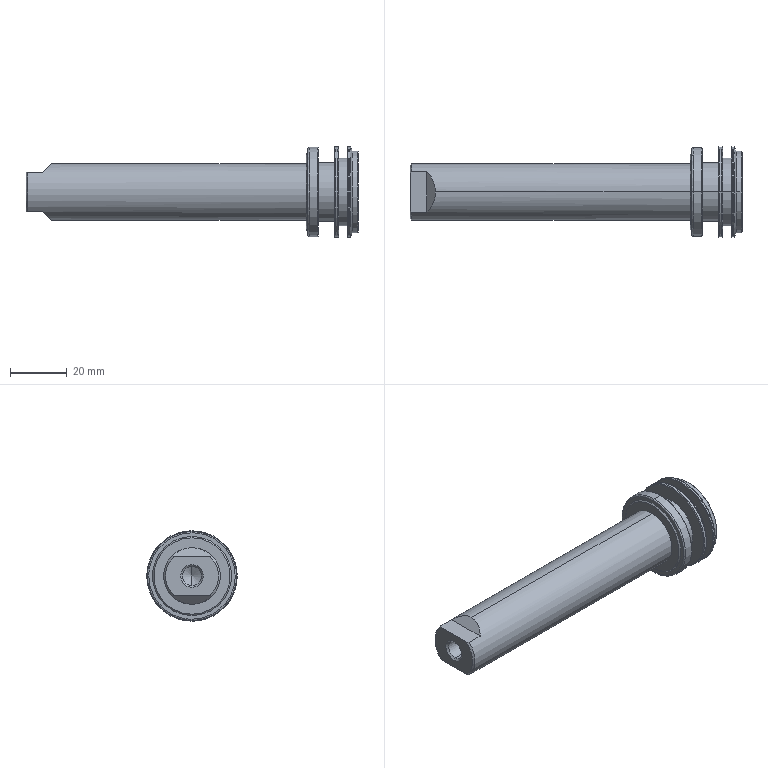Part | SolidWorks | features BaseBody 1 | 1 solid | 52 faces | box 117.5 x 32 x 32 mm | volume 40502 mm3 | cylinder 16 | cone 14 | plane 12 | spline 10 | commonest cylinder face diameters 32 x4 6.647 x2 20 x2 20.82 x2 24 x2 29 x2